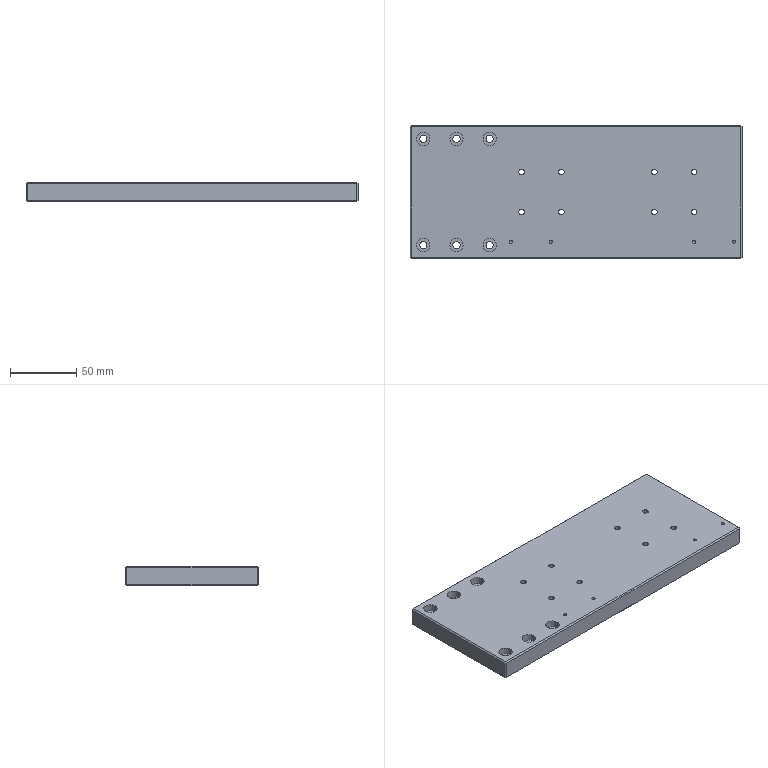Part | STEP file | 06-01 module pad plate | 1 solid | 88 faces | box 250 x 100 x 15 mm | volume 368528 mm3 | cylinder 48 | plane 32 | cone 8 | commonest cylinder face diameters 4.2 x16 5.5 x12 10 x12 2.5 x8